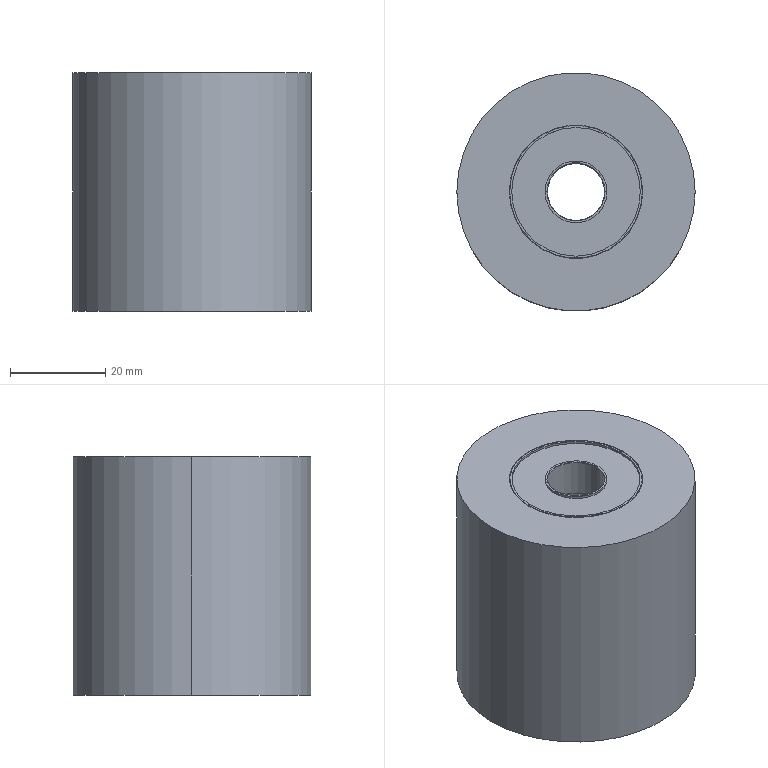Part | STEP file | Copy of QAF43-D50-d12-L50-T5^Clamp mount assembly | 1 solid | 64 faces | box 50 x 50 x 50 mm | volume 80359 mm3 | cylinder 32 | torus 16 | plane 16 | commonest cylinder face diameters 13 x8 27 x8 28 x8 12 x4 23.8 x2 50 x2